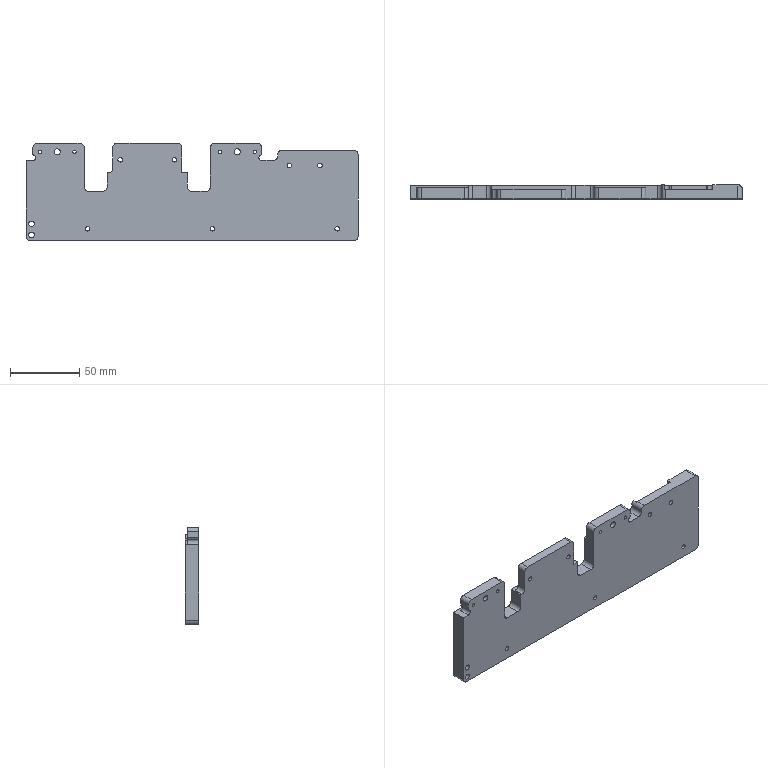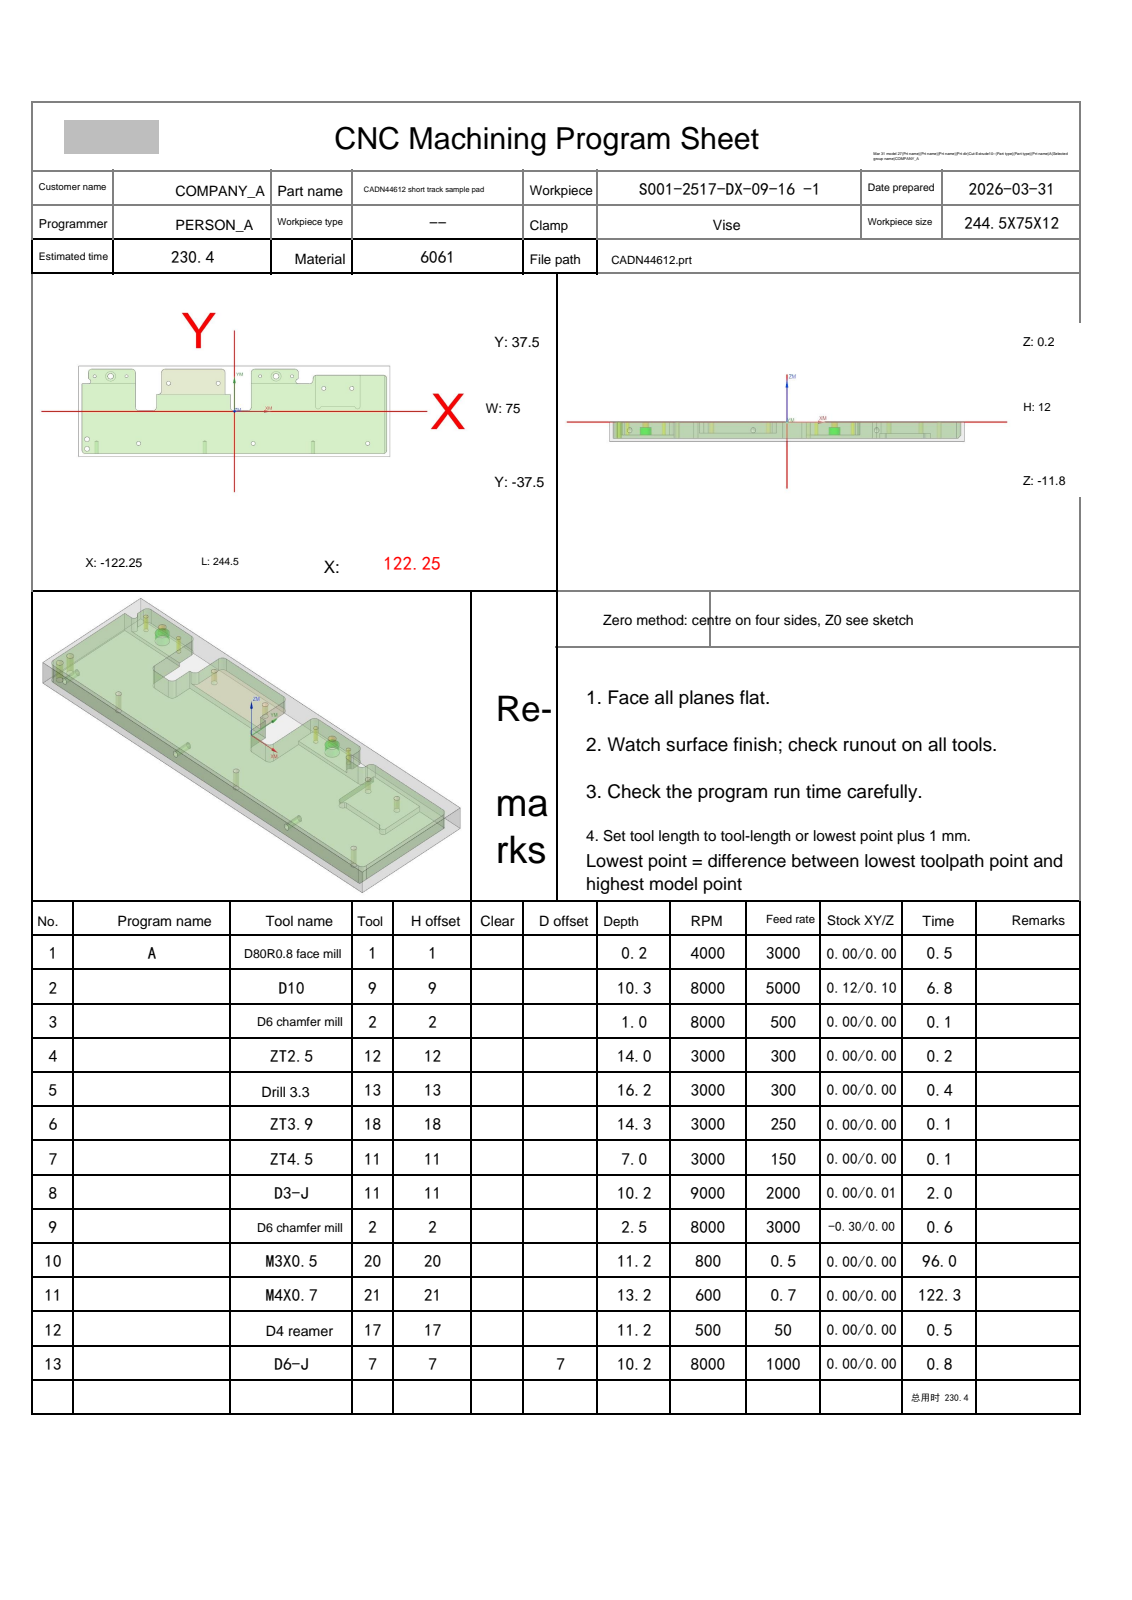NC program | NX | posted by the shop | part box 239.5 x 10 x 70 mm
Lines 2367 to 2413 of 10745:
N5 T13 M06
(Drill 3.3 D=3.3 DR_a=118 H=13)
G00 G90 G54 X104.75 Y-26.5 M03 S3000
G43 H13 Z20.
M08
G98 G83 X104.75 Y-26.5 Z-15.991 R1. F300. Q2.
G98 G83 X92.25 Y19. Z-12.991 R1. Q2.
X70.25
G98 G83 X14.75 Y-26.5 Z-15.991 R1. Q2.
G98 G83 X-12.75 Y23.25 Z-12.791 R1. Q2.
X-51.75
G98 G83 X-75.25 Y-26.5 Z-15.991 R1. Q2.
G80
G00 Z20.
G91 G28 Z0.0
M05
M09
G91 G28 Z0.0
M01
N6 T18 M06
(ZT3.9 D=3.9 DR_a=120 H=18)
G00 G90 G54 X-115.75 Y-23. M03 S3000
G43 H18 Z20.
M08
G98 G83 X-115.75 Y-23. Z-14.126 R1. F250. Q2.
Y-31.
G80
G00 Z20.
G91 G28 Z0.0
M05
M09
G91 G28 Z0.0
M01
N7 T11 M06
(ZT4.5 D=4.5 DR_a=118 H=11)
G00 G90 G54 X32.75 Y29. M03 S3000
G43 H11 Z20.
M08
G98 G83 X32.75 Y29. Z-6.752 R1. F150. Q3.
X-97.25
G80
G00 Z20.
G91 G28 Z0.0
M05
M09
G91 G28 Z0.0
M01